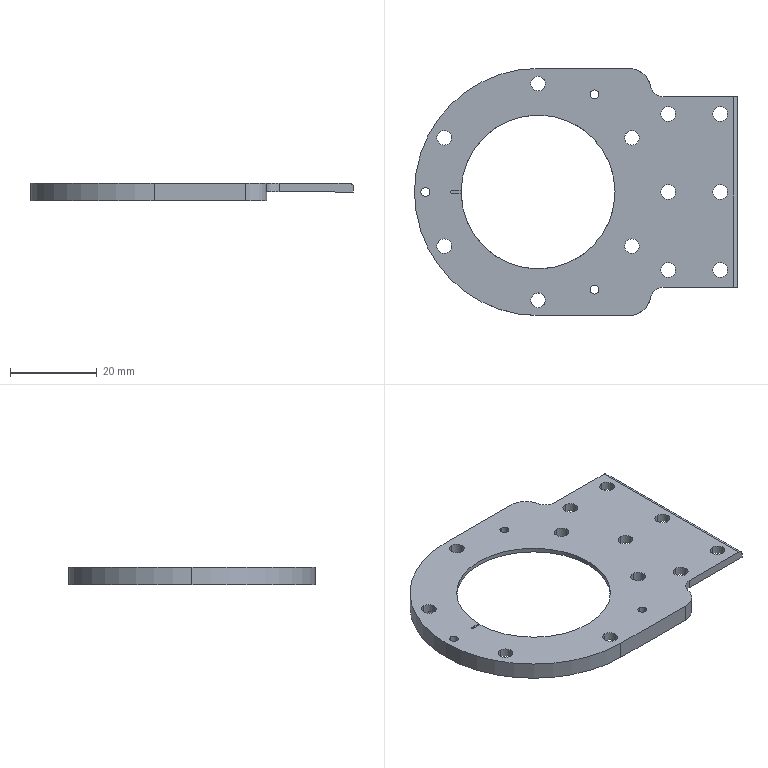NC program | NX | posted with a generic post | part box 74.5 x 57 x 4 mm
Lines 1525 to 3557 of 3557, first 1751 of 2029 lines:
(ZLEVEL_PROFILE_COPY_COPY , TOOL : D10JING)
N2994 T14 M6
N2996 G54
N2998 G17 G0 G90 X-19.345 Y1.822 S9500 M3
N3000 G43 Z30. H14
N3002 Z-3.
N3004 G94 G1 Z-4. F1000.
N3006 X-21. Y0.866
N3008 G3 X-21.5 Y0. R1.
N3010 X-8.75 Y-12.75 R12.75 F1500.
N3012 X-21.5 Y0. R-12.75
N3014 X-21. Y-0.866 R1.
N3016 G1 X-19.345 Y-1.822
N3018 Z-3.
N3020 G0 Z30.
(ZLEVEL_PROFILE_COPY , TOOL : D10JING)
N3022 X44.059 Y23.622
N3024 Z-2.525
N3026 G1 Z-3.525 F1000.
N3028 X42.75 Y22.866
N3030 G3 X42.25 Y22. R1.
N3032 G1 Y-22. F1200.
N3034 G2 X37.25 Y-27. R5.
N3036 G1 X21.617
N3038 G2 X12.25 Y-33.5 R10.
N3040 G1 X-8.75
N3042 G2 X-42.25 Y0. R33.5
N3044 X-8.75 Y33.5 R33.5
N3046 G1 X12.25
N3048 G2 X21.617 Y27. R10.
N3050 G1 X37.25
N3052 G2 X42.25 Y22. R5.
N3054 G1 Y-21.784 Z-3.546
N3056 Y-22.007
N3058 X42.245 Y-22.231
N3060 X42.229 Y-22.454
N3062 X42.204 Y-22.676
N3064 X42.169 Y-22.896
N3066 X42.124 Y-23.115
N3068 X42.069 Y-23.331 Z-3.547
N3070 X42.005 Y-23.545
N3072 X41.931 Y-23.756
N3074 X41.848 Y-23.964
N3076 X41.756 Y-24.167
N3078 X41.655 Y-24.366
N3080 X41.545 Y-24.56
N3082 X41.426 Y-24.75
N3084 X41.299 Y-24.933
N3086 X41.164 Y-25.111 Z-3.548
N3088 X41.021 Y-25.283
N3090 X40.871 Y-25.448
N3092 X40.713 Y-25.607
N3094 X40.549 Y-25.758
N3096 X40.377 Y-25.901
N3098 X40.2 Y-26.037
N3100 X40.017 Y-26.165
N3102 X39.828 Y-26.284
N3104 X39.634 Y-26.395 Z-3.549
N3106 X39.436 Y-26.497
N3108 X39.232 Y-26.59
N3110 X39.025 Y-26.674
N3112 X38.815 Y-26.749
N3114 X38.601 Y-26.814
N3116 X38.385 Y-26.869
N3118 X38.166 Y-26.915
N3120 X37.946 Y-26.951
N3122 X37.724 Y-26.977
N3124 X37.501 Y-26.994 Z-3.55
N3126 X37.278 Y-27.
N3128 X37.055
N3130 X21.641 Z-3.557
N3132 X21.546 Y-27.187
N3134 X21.461 Y-27.393
N3136 X21.372 Y-27.598
N3138 X21.278 Y-27.801 Z-3.558
N3140 X21.18 Y-28.001
N3142 X21.077 Y-28.2
N3144 X20.97 Y-28.396
N3146 X20.858 Y-28.589
N3148 X20.742 Y-28.78
N3150 X20.622 Y-28.969
N3152 X20.498 Y-29.154
N3154 X20.37 Y-29.337
N3156 X20.237 Y-29.517 Z-3.559
N3158 X20.101 Y-29.694
N3160 X19.96 Y-29.868
N3162 X19.816 Y-30.038
N3164 X19.668 Y-30.206
N3166 X19.517 Y-30.37
N3168 X19.361 Y-30.53
N3170 X19.203 Y-30.688
N3172 X19.04 Y-30.841
N3174 X18.875 Y-30.991
N3176 X18.706 Y-31.137 Z-3.56
N3178 X18.533 Y-31.279
N3180 X18.358 Y-31.418
N3182 X18.18 Y-31.552
N3184 X17.998 Y-31.683
N3186 X17.814 Y-31.809
N3188 X17.627 Y-31.931
N3190 X17.438 Y-32.049
N3192 X17.245 Y-32.163
N3194 X17.051 Y-32.272 Z-3.561
N3196 X16.853 Y-32.377
N3198 X16.654 Y-32.478
N3200 X16.452 Y-32.574
N3202 X16.249 Y-32.666
N3204 X16.043 Y-32.753
N3206 X15.835 Y-32.835
N3208 X15.626 Y-32.913
N3210 X15.415 Y-32.986
N3212 X15.202 Y-33.054
N3214 X14.988 Y-33.118 Z-3.562
N3216 X14.772 Y-33.177
N3218 X14.556 Y-33.231
N3220 X14.338 Y-33.28
N3222 X14.119 Y-33.324
N3224 X13.899 Y-33.363
N3226 X13.678 Y-33.398
N3228 X13.457 Y-33.427
N3230 X13.235 Y-33.451
N3232 X13.012 Y-33.471 Z-3.563
N3234 X12.789 Y-33.485
N3236 X12.566 Y-33.495
N3238 X12.343 Y-33.5
N3240 X12.119
N3242 X-8.656 Z-3.573
N3244 X-8.879
N3246 X-9.103 Y-33.498
N3248 X-9.326 Y-33.495
N3250 X-9.549 Y-33.49
N3252 X-9.773 Y-33.484
N3254 X-9.996 Y-33.477 Z-3.574
N3256 X-10.219 Y-33.468
N3258 X-10.442 Y-33.457
N3260 X-10.665 Y-33.445
N3262 X-10.888 Y-33.432
N3264 X-11.111 Y-33.417
N3266 X-11.334 Y-33.4
N3268 X-11.557 Y-33.382
N3270 X-11.779 Y-33.363
N3272 X-12.002 Y-33.342
N3274 X-12.224 Y-33.319 Z-3.575
N3276 X-12.446 Y-33.296
N3278 X-12.668 Y-33.27
N3280 X-12.89 Y-33.243
N3282 X-13.111 Y-33.215
N3284 X-13.333 Y-33.185
N3286 X-13.554 Y-33.154
N3288 X-13.775 Y-33.121
N3290 X-13.995 Y-33.087
N3292 X-14.216 Y-33.051 Z-3.576
N3294 X-14.436 Y-33.014
N3296 X-14.656 Y-32.975
N3298 X-14.876 Y-32.935
N3300 X-15.096 Y-32.894
N3302 X-15.315 Y-32.85
N3304 X-15.534 Y-32.806
N3306 X-15.752 Y-32.76
N3308 X-15.971 Y-32.713
N3310 X-16.189 Y-32.664
N3312 X-16.406 Y-32.613 Z-3.577
N3314 X-16.623 Y-32.562
N3316 X-16.84 Y-32.508
N3318 X-17.057 Y-32.454
N3320 X-17.273 Y-32.398
N3322 X-17.489 Y-32.34
N3324 X-17.705 Y-32.281
N3326 X-17.92 Y-32.221
N3328 X-18.134 Y-32.159
N3330 X-18.348 Y-32.095 Z-3.578
N3332 X-18.562 Y-32.031
N3334 X-18.776 Y-31.965
N3336 X-18.989 Y-31.897
N3338 X-19.201 Y-31.828
N3340 X-19.413 Y-31.758
N3342 X-19.625 Y-31.686
N3344 X-19.836 Y-31.613
N3346 X-20.046 Y-31.538
N3348 X-20.256 Y-31.462 Z-3.579
N3350 X-20.466 Y-31.385
N3352 X-20.675 Y-31.306
N3354 X-20.883 Y-31.226
N3356 X-21.091 Y-31.144
N3358 X-21.299 Y-31.061
N3360 X-21.505 Y-30.977
N3362 X-21.712 Y-30.891
N3364 X-21.917 Y-30.804
N3366 X-22.123 Y-30.715
N3368 X-22.327 Y-30.625 Z-3.58
N3370 X-22.531 Y-30.534
N3372 X-22.734 Y-30.442
N3374 X-22.937 Y-30.348
N3376 X-23.139 Y-30.252
N3378 X-23.34 Y-30.156
N3380 X-23.541 Y-30.058
N3382 X-23.741 Y-29.958
N3384 X-23.941 Y-29.858
N3386 X-24.14 Y-29.756 Z-3.581
N3388 X-24.338 Y-29.653
N3390 X-24.535 Y-29.548
N3392 X-24.732 Y-29.442
N3394 X-24.928 Y-29.335
N3396 X-25.123 Y-29.226
N3398 X-25.317 Y-29.117
N3400 X-25.511 Y-29.005
N3402 X-25.704 Y-28.893
N3404 X-25.897 Y-28.779
N3406 X-26.088 Y-28.664 Z-3.582
N3408 X-26.279 Y-28.548
N3410 X-26.469 Y-28.431
N3412 X-26.658 Y-28.312
N3414 X-26.846 Y-28.192
N3416 X-27.034 Y-28.07
N3418 X-27.221 Y-27.948
N3420 X-27.407 Y-27.824
N3422 X-27.592 Y-27.699
N3424 X-27.776 Y-27.573 Z-3.583
N3426 X-27.96 Y-27.445
N3428 X-28.142 Y-27.317
N3430 X-28.324 Y-27.187
N3432 X-28.505 Y-27.056
N3434 X-28.685 Y-26.923
N3436 X-28.864 Y-26.79
N3438 X-29.042 Y-26.655
N3440 X-29.219 Y-26.519
N3442 X-29.396 Y-26.382 Z-3.584
N3444 X-29.571 Y-26.244
N3446 X-29.746 Y-26.104
N3448 X-29.919 Y-25.964
N3450 X-30.092 Y-25.822
N3452 X-30.264 Y-25.679
N3454 X-30.434 Y-25.535
N3456 X-30.604 Y-25.39
N3458 X-30.773 Y-25.244
N3460 X-30.941 Y-25.096
N3462 X-31.108 Y-24.948 Z-3.585
N3464 X-31.274 Y-24.798
N3466 X-31.438 Y-24.647
N3468 X-31.602 Y-24.495
N3470 X-31.765 Y-24.343
N3472 X-31.927 Y-24.188
N3474 X-32.088 Y-24.033
N3476 X-32.247 Y-23.877
N3478 X-32.406 Y-23.72
N3480 X-32.564 Y-23.562 Z-3.586
N3482 X-32.72 Y-23.402
N3484 X-32.876 Y-23.242
N3486 X-33.03 Y-23.081
N3488 X-33.184 Y-22.918
N3490 X-33.336 Y-22.755
N3492 X-33.487 Y-22.59
N3494 X-33.637 Y-22.425
N3496 X-33.786 Y-22.258
N3498 X-33.934 Y-22.091
N3500 X-34.081 Y-21.923 Z-3.587
N3502 X-34.226 Y-21.753
N3504 X-34.371 Y-21.583
N3506 X-34.514 Y-21.412
N3508 X-34.656 Y-21.239
N3510 X-34.798 Y-21.066
N3512 X-34.937 Y-20.892
N3514 X-35.076 Y-20.717
N3516 X-35.214 Y-20.541
N3518 X-35.35 Y-20.364 Z-3.588
N3520 X-35.485 Y-20.186
N3522 X-35.619 Y-20.007
N3524 X-35.752 Y-19.828
N3526 X-35.884 Y-19.647
N3528 X-36.014 Y-19.466
N3530 X-36.143 Y-19.284
N3532 X-36.271 Y-19.1
N3534 X-36.398 Y-18.917
N3536 X-36.524 Y-18.732 Z-3.589
N3538 X-36.648 Y-18.546
N3540 X-36.771 Y-18.36
N3542 X-36.893 Y-18.172
N3544 X-37.013 Y-17.984
N3546 X-37.133 Y-17.795
N3548 X-37.251 Y-17.606
N3550 X-37.367 Y-17.415
N3552 X-37.483 Y-17.224
N3554 X-37.597 Y-17.032
N3556 X-37.71 Y-16.839 Z-3.59
N3558 X-37.822 Y-16.646
N3560 X-37.932 Y-16.452
N3562 X-38.041 Y-16.257
N3564 X-38.149 Y-16.061
N3566 X-38.255 Y-15.865
N3568 X-38.36 Y-15.668
N3570 X-38.464 Y-15.47
N3572 X-38.567 Y-15.271
N3574 X-38.668 Y-15.072 Z-3.591
N3576 X-38.768 Y-14.872
N3578 X-38.866 Y-14.672
N3580 X-38.963 Y-14.471
N3582 X-39.059 Y-14.269
N3584 X-39.154 Y-14.066
N3586 X-39.247 Y-13.863
N3588 X-39.339 Y-13.66
N3590 X-39.429 Y-13.455
N3592 X-39.518 Y-13.251
N3594 X-39.606 Y-13.045 Z-3.592
N3596 X-39.692 Y-12.839
N3598 X-39.777 Y-12.632
N3600 X-39.86 Y-12.425
N3602 X-39.943 Y-12.218
N3604 X-40.023 Y-12.009
N3606 X-40.103 Y-11.8
N3608 X-40.181 Y-11.591
N3610 X-40.257 Y-11.381
N3612 X-40.333 Y-11.171 Z-3.593
N3614 X-40.406 Y-10.96
N3616 X-40.479 Y-10.749
N3618 X-40.55 Y-10.537
N3620 X-40.619 Y-10.325
N3622 X-40.687 Y-10.112
N3624 X-40.754 Y-9.899
N3626 X-40.819 Y-9.685
N3628 X-40.883 Y-9.471
N3630 X-40.946 Y-9.257 Z-3.594
N3632 X-41.007 Y-9.042
N3634 X-41.066 Y-8.826
N3636 X-41.124 Y-8.611
N3638 X-41.181 Y-8.395
N3640 X-41.236 Y-8.178
N3642 X-41.29 Y-7.961
N3644 X-41.343 Y-7.744
N3646 X-41.394 Y-7.527
N3648 X-41.443 Y-7.309
N3650 X-41.491 Y-7.091 Z-3.595
N3652 X-41.538 Y-6.872
N3654 X-41.583 Y-6.653
N3656 X-41.626 Y-6.434
N3658 X-41.668 Y-6.215
N3660 X-41.709 Y-5.995
N3662 X-41.748 Y-5.775
N3664 X-41.786 Y-5.555
N3666 X-41.822 Y-5.335
N3668 X-41.857 Y-5.114 Z-3.596
N3670 X-41.891 Y-4.893
N3672 X-41.923 Y-4.672
N3674 X-41.953 Y-4.451
N3676 X-41.982 Y-4.229
N3678 X-42.009 Y-4.008
N3680 X-42.035 Y-3.786
N3682 X-42.06 Y-3.564
N3684 X-42.083 Y-3.342
N3686 X-42.104 Y-3.119
N3688 X-42.125 Y-2.897 Z-3.597
N3690 X-42.143 Y-2.674
N3692 X-42.16 Y-2.451
N3694 X-42.176 Y-2.229
N3696 X-42.19 Y-2.006
N3698 X-42.203 Y-1.783
N3700 X-42.214 Y-1.559
N3702 X-42.223 Y-1.336
N3704 X-42.232 Y-1.113
N3706 X-42.238 Y-0.89 Z-3.598
N3708 X-42.243 Y-0.666
N3710 X-42.247 Y-0.443
N3712 X-42.249 Y-0.22
N3714 X-42.25 Y0.004
N3716 X-42.249 Y0.227
N3718 X-42.247 Y0.45
N3720 X-42.243 Y0.674
N3722 X-42.238 Y0.897
N3724 X-42.231 Y1.12 Z-3.599
N3726 X-42.223 Y1.344
N3728 X-42.213 Y1.567
N3730 X-42.202 Y1.79
N3732 X-42.189 Y2.013
N3734 X-42.175 Y2.236
N3736 X-42.16 Y2.459
N3738 X-42.143 Y2.681
N3740 X-42.124 Y2.904
N3742 X-42.104 Y3.127
N3744 X-42.082 Y3.349 Z-3.6
N3746 X-42.059 Y3.571
N3748 X-42.035 Y3.793
N3750 X-42.009 Y4.015
N3752 X-41.981 Y4.237
N3754 X-41.952 Y4.458
N3756 X-41.922 Y4.68
N3758 X-41.89 Y4.901
N3760 X-41.856 Y5.121
N3762 X-41.821 Y5.342 Z-3.601
N3764 X-41.785 Y5.563
N3766 X-41.747 Y5.783
N3768 X-41.708 Y6.003
N3770 X-41.667 Y6.222
N3772 X-41.625 Y6.442
N3774 X-41.581 Y6.661
N3776 X-41.536 Y6.879
N3778 X-41.489 Y7.098
N3780 X-41.441 Y7.316
N3782 X-41.392 Y7.534 Z-3.602
N3784 X-41.341 Y7.751
N3786 X-41.288 Y7.969
N3788 X-41.235 Y8.185
N3790 X-41.179 Y8.402
N3792 X-41.123 Y8.618
N3794 X-41.064 Y8.834
N3796 X-41.005 Y9.049
N3798 X-40.944 Y9.264
N3800 X-40.881 Y9.478 Z-3.603
N3802 X-40.817 Y9.692
N3804 X-40.752 Y9.906
N3806 X-40.685 Y10.119
N3808 X-40.617 Y10.332
N3810 X-40.547 Y10.544
N3812 X-40.476 Y10.756
N3814 X-40.404 Y10.967
N3816 X-40.33 Y11.178
N3818 X-40.255 Y11.388 Z-3.604
N3820 X-40.178 Y11.598
N3822 X-40.1 Y11.807
N3824 X-40.021 Y12.016
N3826 X-39.94 Y12.224
N3828 X-39.858 Y12.432
N3830 X-39.774 Y12.639
N3832 X-39.689 Y12.846
N3834 X-39.603 Y13.052
N3836 X-39.515 Y13.257
N3838 X-39.426 Y13.462 Z-3.605
N3840 X-39.336 Y13.667
N3842 X-39.244 Y13.87
N3844 X-39.151 Y14.073
N3846 X-39.056 Y14.276
N3848 X-38.96 Y14.477
N3850 X-38.863 Y14.678
N3852 X-38.764 Y14.879
N3854 X-38.665 Y15.079
N3856 X-38.563 Y15.278 Z-3.606
N3858 X-38.461 Y15.476
N3860 X-38.357 Y15.674
N3862 X-38.252 Y15.871
N3864 X-38.145 Y16.068
N3866 X-38.037 Y16.263
N3868 X-37.928 Y16.458
N3870 X-37.818 Y16.652
N3872 X-37.706 Y16.846
N3874 X-37.593 Y17.039
N3876 X-37.479 Y17.231 Z-3.607
N3878 X-37.364 Y17.422
N3880 X-37.247 Y17.612
N3882 X-37.129 Y17.802
N3884 X-37.009 Y17.991
N3886 X-36.889 Y18.179
N3888 X-36.767 Y18.366
N3890 X-36.644 Y18.552
N3892 X-36.519 Y18.738
N3894 X-36.394 Y18.923 Z-3.608
N3896 X-36.267 Y19.107
N3898 X-36.139 Y19.29
N3900 X-36.01 Y19.472
N3902 X-35.879 Y19.653
N3904 X-35.748 Y19.834
N3906 X-35.615 Y20.013
N3908 X-35.481 Y20.192
N3910 X-35.346 Y20.37
N3912 X-35.209 Y20.547 Z-3.609
N3914 X-35.072 Y20.723
N3916 X-34.933 Y20.898
N3918 X-34.793 Y21.072
N3920 X-34.652 Y21.245
N3922 X-34.51 Y21.417
N3924 X-34.366 Y21.589
N3926 X-34.222 Y21.759
N3928 X-34.076 Y21.928
N3930 X-33.929 Y22.097
N3932 X-33.781 Y22.264 Z-3.61
N3934 X-33.632 Y22.43
N3936 X-33.482 Y22.596
N3938 X-33.331 Y22.76
N3940 X-33.179 Y22.924
N3942 X-33.025 Y23.086
N3944 X-32.871 Y23.247
N3946 X-32.715 Y23.408
N3948 X-32.558 Y23.567
N3950 X-32.401 Y23.725 Z-3.611
N3952 X-32.242 Y23.882
N3954 X-32.082 Y24.039
N3956 X-31.921 Y24.194
N3958 X-31.76 Y24.348
N3960 X-31.597 Y24.5
N3962 X-31.433 Y24.652
N3964 X-31.268 Y24.803
N3966 X-31.102 Y24.953
N3968 X-30.935 Y25.101
N3970 X-30.767 Y25.248 Z-3.612
N3972 X-30.599 Y25.395
N3974 X-30.429 Y25.54
N3976 X-30.258 Y25.684
N3978 X-30.086 Y25.827
N3980 X-29.913 Y25.968
N3982 X-29.74 Y26.109
N3984 X-29.565 Y26.248
N3986 X-29.39 Y26.387
N3988 X-29.213 Y26.524 Z-3.613
N3990 X-29.036 Y26.659
N3992 X-28.858 Y26.794
N3994 X-28.679 Y26.928
N3996 X-28.499 Y27.06
N3998 X-28.318 Y27.191
N4000 X-28.136 Y27.321
N4002 X-27.953 Y27.45
N4004 X-27.77 Y27.577
N4006 X-27.586 Y27.703 Z-3.614
N4008 X-27.401 Y27.828
N4010 X-27.215 Y27.952
N4012 X-27.028 Y28.074
N4014 X-26.84 Y28.196
N4016 X-26.652 Y28.316
N4018 X-26.462 Y28.434
N4020 X-26.272 Y28.552
N4022 X-26.082 Y28.668
N4024 X-25.89 Y28.783
N4026 X-25.698 Y28.897 Z-3.615
N4028 X-25.505 Y29.009
N4030 X-25.311 Y29.12
N4032 X-25.116 Y29.23
N4034 X-24.921 Y29.338
N4036 X-24.725 Y29.446
N4038 X-24.528 Y29.552
N4040 X-24.331 Y29.656
N4042 X-24.133 Y29.759
N4044 X-23.934 Y29.861 Z-3.616
N4046 X-23.735 Y29.962
N4048 X-23.535 Y30.061
N4050 X-23.334 Y30.159
N4052 X-23.132 Y30.256
N4054 X-22.93 Y30.351
N4056 X-22.728 Y30.445
N4058 X-22.524 Y30.537
N4060 X-22.32 Y30.628
N4062 X-22.116 Y30.718
N4064 X-21.911 Y30.807 Z-3.617
N4066 X-21.705 Y30.894
N4068 X-21.499 Y30.979
N4070 X-21.292 Y31.064
N4072 X-21.084 Y31.147
N4074 X-20.876 Y31.228
N4076 X-20.668 Y31.308
N4078 X-20.459 Y31.387
N4080 X-20.249 Y31.465
N4082 X-20.039 Y31.541 Z-3.618
N4084 X-19.829 Y31.615
N4086 X-19.618 Y31.688
N4088 X-19.406 Y31.76
N4090 X-19.194 Y31.83
N4092 X-18.982 Y31.899
N4094 X-18.769 Y31.967
N4096 X-18.555 Y32.033
N4098 X-18.341 Y32.098
N4100 X-18.127 Y32.161 Z-3.619
N4102 X-17.912 Y32.223
N4104 X-17.697 Y32.283
N4106 X-17.482 Y32.342
N4108 X-17.266 Y32.399
N4110 X-17.05 Y32.456
N4112 X-16.833 Y32.51
N4114 X-16.616 Y32.563
N4116 X-16.399 Y32.615
N4118 X-16.181 Y32.665
N4120 X-15.963 Y32.714 Z-3.62
N4122 X-15.745 Y32.762
N4124 X-15.526 Y32.807
N4126 X-15.307 Y32.852
N4128 X-15.088 Y32.895
N4130 X-14.869 Y32.936
N4132 X-14.649 Y32.977
N4134 X-14.429 Y33.015
N4136 X-14.209 Y33.052
N4138 X-13.988 Y33.088 Z-3.621
N4140 X-13.767 Y33.122
N4142 X-13.546 Y33.155
N4144 X-13.325 Y33.186
N4146 X-13.104 Y33.216
N4148 X-12.882 Y33.244
N4150 X-12.66 Y33.271
N4152 X-12.439 Y33.296
N4154 X-12.216 Y33.32
N4156 X-11.994 Y33.343
N4158 X-11.772 Y33.363 Z-3.622
N4160 X-11.549 Y33.383
N4162 X-11.327 Y33.401
N4164 X-11.104 Y33.417
N4166 X-10.881 Y33.432
N4168 X-10.658 Y33.446
N4170 X-10.435 Y33.458
N4172 X-10.212 Y33.468
N4174 X-9.988 Y33.477
N4176 X-9.765 Y33.485 Z-3.623
N4178 X-9.542 Y33.491
N4180 X-9.319 Y33.495
N4182 X-9.095 Y33.498
N4184 X-8.872 Y33.5
N4186 X-8.648
N4188 X12.127 Z-3.633
N4190 X12.35
N4192 X12.573 Y33.495
N4194 X12.797 Y33.485
N4196 X13.019 Y33.47
N4198 X13.242 Y33.451 Z-3.634
N4200 X13.464 Y33.426
N4202 X13.685 Y33.396
N4204 X13.906 Y33.362
N4206 X14.126 Y33.322
N4208 X14.345 Y33.278
N4210 X14.563 Y33.229
N4212 X14.78 Y33.175
N4214 X14.995 Y33.116
N4216 X15.209 Y33.052
N4218 X15.422 Y32.984 Z-3.635
N4220 X15.633 Y32.91
N4222 X15.842 Y32.833
N4224 X16.05 Y32.75
N4226 X16.255 Y32.663
N4228 X16.459 Y32.571
N4230 X16.661 Y32.475
N4232 X16.86 Y32.374
N4234 X17.057 Y32.269
N4236 X17.252 Y32.159 Z-3.636
N4238 X17.444 Y32.045
N4240 X17.633 Y31.927
N4242 X17.82 Y31.805
N4244 X18.004 Y31.678
N4246 X18.186 Y31.548
N4248 X18.364 Y31.413
N4250 X18.539 Y31.275
N4252 X18.711 Y31.132
N4254 X18.88 Y30.986
N4256 X19.046 Y30.836 Z-3.637
N4258 X19.208 Y30.682
N4260 X19.367 Y30.525
N4262 X19.522 Y30.364
N4264 X19.673 Y30.2
N4266 X19.821 Y30.033
N4268 X19.965 Y29.862
N4270 X20.105 Y29.688
N4272 X20.242 Y29.511
N4274 X20.374 Y29.331 Z-3.638
N4276 X20.502 Y29.148
N4278 X20.626 Y28.963
N4280 X20.746 Y28.774
N4282 X20.862 Y28.583
N4284 X20.973 Y28.389
N4286 X21.08 Y28.193
N4288 X21.183 Y27.995
N4290 X21.281 Y27.794
N4292 X21.375 Y27.591 Z-3.639
N4294 X21.464 Y27.387
N4296 X21.548 Y27.18
N4298 X21.648 Y27.
N4300 X37.062 Z-3.646
N4302 X37.285
N4304 X37.509 Y26.993
N4306 X37.731 Y26.977
N4308 X37.953 Y26.95 Z-3.647
N4310 X38.174 Y26.914
N4312 X38.392 Y26.868
N4314 X38.608 Y26.812
N4316 X38.822 Y26.746
N4318 X39.032 Y26.672
N4320 X39.239 Y26.587
N4322 X39.442 Y26.494
N4324 X39.641 Y26.391
N4326 X39.834 Y26.28 Z-3.648
N4328 X40.023 Y26.161
N4330 X40.206 Y26.033
N4332 X40.383 Y25.897
N4334 X40.554 Y25.753
N4336 X40.718 Y25.601
N4338 X40.876 Y25.443
N4340 X41.026 Y25.277
N4342 X41.169 Y25.106
N4344 X41.303 Y24.927 Z-3.649
N4346 X41.43 Y24.744
N4348 X41.548 Y24.554
N4350 X41.658 Y24.36
N4352 X41.759 Y24.16
N4354 X41.851 Y23.957
N4356 X41.934 Y23.749
N4358 X42.007 Y23.538
N4360 X42.071 Y23.324
N4362 X42.126 Y23.108
N4364 X42.17 Y22.889 Z-3.65
N4366 X42.205 Y22.668
N4368 X42.23 Y22.446
N4370 X42.245 Y22.223
N4372 X42.25 Y22.
N4374 Y-21.784 Z-3.671
N4376 Y-22.007
N4378 X42.245 Y-22.231
N4380 X42.229 Y-22.454
N4382 X42.204 Y-22.676
N4384 X42.169 Y-22.896
N4386 X42.124 Y-23.115
N4388 X42.069 Y-23.331 Z-3.672
N4390 X42.005 Y-23.545
N4392 X41.931 Y-23.756
N4394 X41.848 Y-23.964
N4396 X41.756 Y-24.167
N4398 X41.655 Y-24.366
N4400 X41.545 Y-24.56
N4402 X41.426 Y-24.75
N4404 X41.299 Y-24.933
N4406 X41.164 Y-25.111 Z-3.673
N4408 X41.021 Y-25.283
N4410 X40.871 Y-25.448
N4412 X40.713 Y-25.607
N4414 X40.549 Y-25.758
N4416 X40.377 Y-25.901
N4418 X40.2 Y-26.037
N4420 X40.017 Y-26.165
N4422 X39.828 Y-26.284
N4424 X39.634 Y-26.395 Z-3.674
N4426 X39.436 Y-26.497
N4428 X39.232 Y-26.59
N4430 X39.025 Y-26.674
N4432 X38.815 Y-26.749
N4434 X38.601 Y-26.814
N4436 X38.385 Y-26.869
N4438 X38.166 Y-26.915
N4440 X37.946 Y-26.951
N4442 X37.724 Y-26.977
N4444 X37.501 Y-26.994 Z-3.675
N4446 X37.278 Y-27.
N4448 X37.055
N4450 X21.641 Z-3.682
N4452 X21.546 Y-27.187
N4454 X21.461 Y-27.393
N4456 X21.372 Y-27.598
N4458 X21.278 Y-27.801 Z-3.683
N4460 X21.18 Y-28.001
N4462 X21.077 Y-28.2
N4464 X20.97 Y-28.396
N4466 X20.858 Y-28.589
N4468 X20.742 Y-28.78
N4470 X20.622 Y-28.969
N4472 X20.498 Y-29.154
N4474 X20.37 Y-29.337
N4476 X20.237 Y-29.517 Z-3.684
N4478 X20.101 Y-29.694
N4480 X19.96 Y-29.868
N4482 X19.816 Y-30.038
N4484 X19.668 Y-30.206
N4486 X19.517 Y-30.37
N4488 X19.361 Y-30.53
N4490 X19.203 Y-30.688
N4492 X19.04 Y-30.841
N4494 X18.875 Y-30.991
N4496 X18.706 Y-31.137 Z-3.685
N4498 X18.533 Y-31.279
N4500 X18.358 Y-31.418
N4502 X18.18 Y-31.552
N4504 X17.998 Y-31.683
N4506 X17.814 Y-31.809
N4508 X17.627 Y-31.931
N4510 X17.438 Y-32.049
N4512 X17.245 Y-32.163
N4514 X17.051 Y-32.272 Z-3.686
N4516 X16.853 Y-32.377
N4518 X16.654 Y-32.478
N4520 X16.452 Y-32.574
N4522 X16.249 Y-32.666
N4524 X16.043 Y-32.753
N4526 X15.835 Y-32.835
N4528 X15.626 Y-32.913
N4530 X15.415 Y-32.986
N4532 X15.202 Y-33.054
N4534 X14.988 Y-33.118 Z-3.687
N4536 X14.772 Y-33.177
N4538 X14.556 Y-33.231
N4540 X14.338 Y-33.28
N4542 X14.119 Y-33.324
N4544 X13.899 Y-33.363
N4546 X13.678 Y-33.398
N4548 X13.457 Y-33.427
N4550 X13.235 Y-33.451
N4552 X13.012 Y-33.471 Z-3.688
N4554 X12.789 Y-33.485
N4556 X12.566 Y-33.495
N4558 X12.343 Y-33.5
N4560 X12.119
N4562 X-8.656 Z-3.698
N4564 X-8.879
N4566 X-9.103 Y-33.498
N4568 X-9.326 Y-33.495
N4570 X-9.549 Y-33.49
N4572 X-9.773 Y-33.484
N4574 X-9.996 Y-33.477 Z-3.699
N4576 X-10.219 Y-33.468
N4578 X-10.442 Y-33.457
N4580 X-10.665 Y-33.445
N4582 X-10.888 Y-33.432
N4584 X-11.111 Y-33.417
N4586 X-11.334 Y-33.4
N4588 X-11.557 Y-33.382
N4590 X-11.779 Y-33.363
N4592 X-12.002 Y-33.342
N4594 X-12.224 Y-33.319 Z-3.7
N4596 X-12.446 Y-33.296
N4598 X-12.668 Y-33.27
N4600 X-12.89 Y-33.243
N4602 X-13.111 Y-33.215
N4604 X-13.333 Y-33.185
N4606 X-13.554 Y-33.154
N4608 X-13.775 Y-33.121
N4610 X-13.995 Y-33.087
N4612 X-14.216 Y-33.051 Z-3.701
N4614 X-14.436 Y-33.014
N4616 X-14.656 Y-32.975
N4618 X-14.876 Y-32.935
N4620 X-15.096 Y-32.894
N4622 X-15.315 Y-32.85
N4624 X-15.534 Y-32.806
N4626 X-15.752 Y-32.76
N4628 X-15.971 Y-32.713
N4630 X-16.189 Y-32.664
N4632 X-16.406 Y-32.613 Z-3.702
N4634 X-16.623 Y-32.562
N4636 X-16.84 Y-32.508
N4638 X-17.057 Y-32.454
N4640 X-17.273 Y-32.398
N4642 X-17.489 Y-32.34
N4644 X-17.705 Y-32.281
N4646 X-17.92 Y-32.221
N4648 X-18.134 Y-32.159
N4650 X-18.348 Y-32.095 Z-3.703
N4652 X-18.562 Y-32.031
N4654 X-18.776 Y-31.965
N4656 X-18.989 Y-31.897
N4658 X-19.201 Y-31.828
N4660 X-19.413 Y-31.758
N4662 X-19.625 Y-31.686
N4664 X-19.836 Y-31.613
N4666 X-20.046 Y-31.538
N4668 X-20.256 Y-31.462 Z-3.704
N4670 X-20.466 Y-31.385
N4672 X-20.675 Y-31.306
N4674 X-20.883 Y-31.226
N4676 X-21.091 Y-31.144
N4678 X-21.299 Y-31.061
N4680 X-21.505 Y-30.977
N4682 X-21.712 Y-30.891
N4684 X-21.917 Y-30.804
N4686 X-22.123 Y-30.715
N4688 X-22.327 Y-30.625 Z-3.705
N4690 X-22.531 Y-30.534
N4692 X-22.734 Y-30.442
N4694 X-22.937 Y-30.348
N4696 X-23.139 Y-30.252
N4698 X-23.34 Y-30.156
N4700 X-23.541 Y-30.058
N4702 X-23.741 Y-29.958
N4704 X-23.941 Y-29.858
N4706 X-24.14 Y-29.756 Z-3.706
N4708 X-24.338 Y-29.653
N4710 X-24.535 Y-29.548
N4712 X-24.732 Y-29.442
N4714 X-24.928 Y-29.335
N4716 X-25.123 Y-29.226
N4718 X-25.317 Y-29.117
N4720 X-25.511 Y-29.005
N4722 X-25.704 Y-28.893
N4724 X-25.897 Y-28.779
N4726 X-26.088 Y-28.664 Z-3.707
N4728 X-26.279 Y-28.548
N4730 X-26.469 Y-28.431
N4732 X-26.658 Y-28.312
N4734 X-26.846 Y-28.192
N4736 X-27.034 Y-28.07
N4738 X-27.221 Y-27.948
N4740 X-27.407 Y-27.824
N4742 X-27.592 Y-27.699
N4744 X-27.776 Y-27.573 Z-3.708
N4746 X-27.96 Y-27.445
N4748 X-28.142 Y-27.317
N4750 X-28.324 Y-27.187
N4752 X-28.505 Y-27.056
N4754 X-28.685 Y-26.923
N4756 X-28.864 Y-26.79
N4758 X-29.042 Y-26.655
N4760 X-29.219 Y-26.519
N4762 X-29.396 Y-26.382 Z-3.709
N4764 X-29.571 Y-26.244
N4766 X-29.746 Y-26.104
N4768 X-29.919 Y-25.964
N4770 X-30.092 Y-25.822
N4772 X-30.264 Y-25.679
N4774 X-30.434 Y-25.535
N4776 X-30.604 Y-25.39
N4778 X-30.773 Y-25.244
N4780 X-30.941 Y-25.096
N4782 X-31.108 Y-24.948 Z-3.71
N4784 X-31.274 Y-24.798
N4786 X-31.438 Y-24.647
N4788 X-31.602 Y-24.495
N4790 X-31.765 Y-24.343
N4792 X-31.927 Y-24.188
N4794 X-32.088 Y-24.033
N4796 X-32.247 Y-23.877
N4798 X-32.406 Y-23.72
N4800 X-32.564 Y-23.562 Z-3.711
N4802 X-32.72 Y-23.402
N4804 X-32.876 Y-23.242
N4806 X-33.03 Y-23.081
N4808 X-33.184 Y-22.918
N4810 X-33.336 Y-22.755
N4812 X-33.487 Y-22.59
N4814 X-33.637 Y-22.425
N4816 X-33.786 Y-22.258
N4818 X-33.934 Y-22.091
N4820 X-34.081 Y-21.923 Z-3.712
N4822 X-34.226 Y-21.753
N4824 X-34.371 Y-21.583
N4826 X-34.514 Y-21.412
N4828 X-34.656 Y-21.239
N4830 X-34.798 Y-21.066
N4832 X-34.937 Y-20.892
N4834 X-35.076 Y-20.717
N4836 X-35.214 Y-20.541
N4838 X-35.35 Y-20.364 Z-3.713
N4840 X-35.485 Y-20.186
N4842 X-35.619 Y-20.007
N4844 X-35.752 Y-19.828
N4846 X-35.884 Y-19.647
N4848 X-36.014 Y-19.466
N4850 X-36.143 Y-19.284
N4852 X-36.271 Y-19.1
N4854 X-36.398 Y-18.917
N4856 X-36.524 Y-18.732 Z-3.714
N4858 X-36.648 Y-18.546
N4860 X-36.771 Y-18.36
N4862 X-36.893 Y-18.172
N4864 X-37.013 Y-17.984
N4866 X-37.133 Y-17.795
N4868 X-37.251 Y-17.606
N4870 X-37.367 Y-17.415
N4872 X-37.483 Y-17.224
N4874 X-37.597 Y-17.032
N4876 X-37.71 Y-16.839 Z-3.715
N4878 X-37.822 Y-16.646
N4880 X-37.932 Y-16.452
N4882 X-38.041 Y-16.257
N4884 X-38.149 Y-16.061
N4886 X-38.255 Y-15.865
N4888 X-38.36 Y-15.668
N4890 X-38.464 Y-15.47
N4892 X-38.567 Y-15.271
N4894 X-38.668 Y-15.072 Z-3.716
N4896 X-38.768 Y-14.872
N4898 X-38.866 Y-14.672
N4900 X-38.963 Y-14.471
N4902 X-39.059 Y-14.269
N4904 X-39.154 Y-14.066
N4906 X-39.247 Y-13.863
N4908 X-39.339 Y-13.66
N4910 X-39.429 Y-13.455
N4912 X-39.518 Y-13.251
N4914 X-39.606 Y-13.045 Z-3.717
N4916 X-39.692 Y-12.839
N4918 X-39.777 Y-12.632
N4920 X-39.86 Y-12.425
N4922 X-39.943 Y-12.218
N4924 X-40.023 Y-12.009
N4926 X-40.103 Y-11.8
N4928 X-40.181 Y-11.591
N4930 X-40.257 Y-11.381
N4932 X-40.333 Y-11.171 Z-3.718
N4934 X-40.406 Y-10.96
N4936 X-40.479 Y-10.749
N4938 X-40.55 Y-10.537
N4940 X-40.619 Y-10.325
N4942 X-40.687 Y-10.112
N4944 X-40.754 Y-9.899
N4946 X-40.819 Y-9.685
N4948 X-40.883 Y-9.471
N4950 X-40.946 Y-9.257 Z-3.719
N4952 X-41.007 Y-9.042
N4954 X-41.066 Y-8.826
N4956 X-41.124 Y-8.611
N4958 X-41.181 Y-8.395
N4960 X-41.236 Y-8.178
N4962 X-41.29 Y-7.961
N4964 X-41.343 Y-7.744
N4966 X-41.394 Y-7.527
N4968 X-41.443 Y-7.309
N4970 X-41.491 Y-7.091 Z-3.72
N4972 X-41.538 Y-6.872
N4974 X-41.583 Y-6.653
N4976 X-41.626 Y-6.434
N4978 X-41.668 Y-6.215
N4980 X-41.709 Y-5.995
N4982 X-41.748 Y-5.775
N4984 X-41.786 Y-5.555
N4986 X-41.822 Y-5.335
N4988 X-41.857 Y-5.114 Z-3.721
N4990 X-41.891 Y-4.893
N4992 X-41.923 Y-4.672
N4994 X-41.953 Y-4.451
N4996 X-41.982 Y-4.229
N4998 X-42.009 Y-4.008
N5000 X-42.035 Y-3.786
N5002 X-42.06 Y-3.564
N5004 X-42.083 Y-3.342
N5006 X-42.104 Y-3.119
N5008 X-42.125 Y-2.897 Z-3.722
N5010 X-42.143 Y-2.674
N5012 X-42.16 Y-2.451
N5014 X-42.176 Y-2.229
N5016 X-42.19 Y-2.006
N5018 X-42.203 Y-1.783
N5020 X-42.214 Y-1.559
N5022 X-42.223 Y-1.336
N5024 X-42.232 Y-1.113
N5026 X-42.238 Y-0.89 Z-3.723
N5028 X-42.243 Y-0.666
N5030 X-42.247 Y-0.443
N5032 X-42.249 Y-0.22
N5034 X-42.25 Y0.004
N5036 X-42.249 Y0.227
N5038 X-42.247 Y0.45
N5040 X-42.243 Y0.674
N5042 X-42.238 Y0.897
N5044 X-42.231 Y1.12 Z-3.724
N5046 X-42.223 Y1.344
N5048 X-42.213 Y1.567
N5050 X-42.202 Y1.79
N5052 X-42.189 Y2.013
N5054 X-42.175 Y2.236
N5056 X-42.16 Y2.459
N5058 X-42.143 Y2.681
N5060 X-42.124 Y2.904
N5062 X-42.104 Y3.127
N5064 X-42.082 Y3.349 Z-3.725
N5066 X-42.059 Y3.571
N5068 X-42.035 Y3.793
N5070 X-42.009 Y4.015
N5072 X-41.981 Y4.237
N5074 X-41.952 Y4.458
N5076 X-41.922 Y4.68
N5078 X-41.89 Y4.901
N5080 X-41.856 Y5.121
N5082 X-41.821 Y5.342 Z-3.726
N5084 X-41.785 Y5.563
N5086 X-41.747 Y5.783
N5088 X-41.708 Y6.003
N5090 X-41.667 Y6.222
N5092 X-41.625 Y6.442
N5094 X-41.581 Y6.661
N5096 X-41.536 Y6.879
N5098 X-41.489 Y7.098
N5100 X-41.441 Y7.316
N5102 X-41.392 Y7.534 Z-3.727
N5104 X-41.341 Y7.751
N5106 X-41.288 Y7.969
N5108 X-41.235 Y8.185
N5110 X-41.179 Y8.402
N5112 X-41.123 Y8.618
N5114 X-41.064 Y8.834
N5116 X-41.005 Y9.049
N5118 X-40.944 Y9.264
N5120 X-40.881 Y9.478 Z-3.728
N5122 X-40.817 Y9.692
N5124 X-40.752 Y9.906
N5126 X-40.685 Y10.119
N5128 X-40.617 Y10.332
N5130 X-40.547 Y10.544
N5132 X-40.476 Y10.756
N5134 X-40.404 Y10.967
N5136 X-40.33 Y11.178
N5138 X-40.255 Y11.388 Z-3.729
N5140 X-40.178 Y11.598
N5142 X-40.1 Y11.807
N5144 X-40.021 Y12.016
N5146 X-39.94 Y12.224
N5148 X-39.858 Y12.432
N5150 X-39.774 Y12.639
N5152 X-39.689 Y12.846
N5154 X-39.603 Y13.052
N5156 X-39.515 Y13.257
N5158 X-39.426 Y13.462 Z-3.73
N5160 X-39.336 Y13.667
N5162 X-39.244 Y13.87
N5164 X-39.151 Y14.073
N5166 X-39.056 Y14.276
N5168 X-38.96 Y14.477
N5170 X-38.863 Y14.678
N5172 X-38.764 Y14.879
N5174 X-38.665 Y15.079
N5176 X-38.563 Y15.278 Z-3.731
N5178 X-38.461 Y15.476
N5180 X-38.357 Y15.674
N5182 X-38.252 Y15.871
N5184 X-38.145 Y16.068
N5186 X-38.037 Y16.263
N5188 X-37.928 Y16.458
N5190 X-37.818 Y16.652
N5192 X-37.706 Y16.846
N5194 X-37.593 Y17.039
N5196 X-37.479 Y17.231 Z-3.732
N5198 X-37.364 Y17.422
N5200 X-37.247 Y17.612
N5202 X-37.129 Y17.802
N5204 X-37.009 Y17.991
N5206 X-36.889 Y18.179
N5208 X-36.767 Y18.366
N5210 X-36.644 Y18.552
N5212 X-36.519 Y18.738
N5214 X-36.394 Y18.923 Z-3.733
N5216 X-36.267 Y19.107
N5218 X-36.139 Y19.29
N5220 X-36.01 Y19.472
N5222 X-35.879 Y19.653
N5224 X-35.748 Y19.834
N5226 X-35.615 Y20.013
N5228 X-35.481 Y20.192
N5230 X-35.346 Y20.37
N5232 X-35.209 Y20.547 Z-3.734
N5234 X-35.072 Y20.723
N5236 X-34.933 Y20.898
N5238 X-34.793 Y21.072
N5240 X-34.652 Y21.245
N5242 X-34.51 Y21.417
N5244 X-34.366 Y21.589
N5246 X-34.222 Y21.759
N5248 X-34.076 Y21.928
N5250 X-33.929 Y22.097
N5252 X-33.781 Y22.264 Z-3.735
N5254 X-33.632 Y22.43
N5256 X-33.482 Y22.596
N5258 X-33.331 Y22.76
N5260 X-33.179 Y22.924
N5262 X-33.025 Y23.086
N5264 X-32.871 Y23.247
N5266 X-32.715 Y23.408
N5268 X-32.558 Y23.567
N5270 X-32.401 Y23.725 Z-3.736
N5272 X-32.242 Y23.882
N5274 X-32.082 Y24.039
N5276 X-31.921 Y24.194
N5278 X-31.76 Y24.348
N5280 X-31.597 Y24.5
N5282 X-31.433 Y24.652
N5284 X-31.268 Y24.803
N5286 X-31.102 Y24.953
N5288 X-30.935 Y25.101
N5290 X-30.767 Y25.248 Z-3.737
N5292 X-30.599 Y25.395
N5294 X-30.429 Y25.54
N5296 X-30.258 Y25.684
N5298 X-30.086 Y25.827
N5300 X-29.913 Y25.968
N5302 X-29.74 Y26.109
N5304 X-29.565 Y26.248
N5306 X-29.39 Y26.387
N5308 X-29.213 Y26.524 Z-3.738
N5310 X-29.036 Y26.659
N5312 X-28.858 Y26.794
N5314 X-28.679 Y26.928
N5316 X-28.499 Y27.06
N5318 X-28.318 Y27.191
N5320 X-28.136 Y27.321
N5322 X-27.953 Y27.45
N5324 X-27.77 Y27.577
N5326 X-27.586 Y27.703 Z-3.739
N5328 X-27.401 Y27.828
N5330 X-27.215 Y27.952
N5332 X-27.028 Y28.074
N5334 X-26.84 Y28.196
N5336 X-26.652 Y28.316
N5338 X-26.462 Y28.434
N5340 X-26.272 Y28.552
N5342 X-26.082 Y28.668
N5344 X-25.89 Y28.783
N5346 X-25.698 Y28.897 Z-3.74
N5348 X-25.505 Y29.009
N5350 X-25.311 Y29.12
N5352 X-25.116 Y29.23
N5354 X-24.921 Y29.338
N5356 X-24.725 Y29.446
N5358 X-24.528 Y29.552
N5360 X-24.331 Y29.656
N5362 X-24.133 Y29.759
N5364 X-23.934 Y29.861 Z-3.741
N5366 X-23.735 Y29.962
N5368 X-23.535 Y30.061
N5370 X-23.334 Y30.159
N5372 X-23.132 Y30.256
N5374 X-22.93 Y30.351
N5376 X-22.728 Y30.445
N5378 X-22.524 Y30.537
N5380 X-22.32 Y30.628
N5382 X-22.116 Y30.718
N5384 X-21.911 Y30.807 Z-3.742
N5386 X-21.705 Y30.894
N5388 X-21.499 Y30.979
N5390 X-21.292 Y31.064
N5392 X-21.084 Y31.147
N5394 X-20.876 Y31.228
N5396 X-20.668 Y31.308
N5398 X-20.459 Y31.387
N5400 X-20.249 Y31.465
N5402 X-20.039 Y31.541 Z-3.743
N5404 X-19.829 Y31.615
N5406 X-19.618 Y31.688
N5408 X-19.406 Y31.76
N5410 X-19.194 Y31.83
N5412 X-18.982 Y31.899
N5414 X-18.769 Y31.967
N5416 X-18.555 Y32.033
N5418 X-18.341 Y32.098
N5420 X-18.127 Y32.161 Z-3.744
N5422 X-17.912 Y32.223
N5424 X-17.697 Y32.283
N5426 X-17.482 Y32.342
N5428 X-17.266 Y32.399
N5430 X-17.05 Y32.456
N5432 X-16.833 Y32.51
N5434 X-16.616 Y32.563
N5436 X-16.399 Y32.615
N5438 X-16.181 Y32.665
N5440 X-15.963 Y32.714 Z-3.745
N5442 X-15.745 Y32.762
N5444 X-15.526 Y32.807
N5446 X-15.307 Y32.852
N5448 X-15.088 Y32.895
N5450 X-14.869 Y32.936
N5452 X-14.649 Y32.977
N5454 X-14.429 Y33.015
N5456 X-14.209 Y33.052
N5458 X-13.988 Y33.088 Z-3.746
N5460 X-13.767 Y33.122
N5462 X-13.546 Y33.155
N5464 X-13.325 Y33.186
N5466 X-13.104 Y33.216
N5468 X-12.882 Y33.244
N5470 X-12.66 Y33.271
N5472 X-12.439 Y33.296
N5474 X-12.216 Y33.32
N5476 X-11.994 Y33.343
N5478 X-11.772 Y33.363 Z-3.747
N5480 X-11.549 Y33.383
N5482 X-11.327 Y33.401
N5484 X-11.104 Y33.417
N5486 X-10.881 Y33.432
N5488 X-10.658 Y33.446
N5490 X-10.435 Y33.458
N5492 X-10.212 Y33.468
N5494 X-9.988 Y33.477
N5496 X-9.765 Y33.485 Z-3.748
N5498 X-9.542 Y33.491
N5500 X-9.319 Y33.495
N5502 X-9.095 Y33.498
N5504 X-8.872 Y33.5
N5506 X-8.648
N5508 X12.127 Z-3.758
N5510 X12.35
N5512 X12.573 Y33.495
N5514 X12.797 Y33.485
N5516 X13.019 Y33.47
N5518 X13.242 Y33.451 Z-3.759
N5520 X13.464 Y33.426
N5522 X13.685 Y33.396
N5524 X13.906 Y33.362
N5526 X14.126 Y33.322
N5528 X14.345 Y33.278
N5530 X14.563 Y33.229
N5532 X14.78 Y33.175
N5534 X14.995 Y33.116
N5536 X15.209 Y33.052
N5538 X15.422 Y32.984 Z-3.76
N5540 X15.633 Y32.91
N5542 X15.842 Y32.833
N5544 X16.05 Y32.75
N5546 X16.255 Y32.663
N5548 X16.459 Y32.571
N5550 X16.661 Y32.475
N5552 X16.86 Y32.374
N5554 X17.057 Y32.269
N5556 X17.252 Y32.159 Z-3.761
N5558 X17.444 Y32.045
N5560 X17.633 Y31.927
N5562 X17.82 Y31.805
N5564 X18.004 Y31.678
N5566 X18.186 Y31.548
N5568 X18.364 Y31.413
N5570 X18.539 Y31.275
N5572 X18.711 Y31.132
N5574 X18.88 Y30.986
N5576 X19.046 Y30.836 Z-3.762
N5578 X19.208 Y30.682
N5580 X19.367 Y30.525
N5582 X19.522 Y30.364
N5584 X19.673 Y30.2
N5586 X19.821 Y30.033
N5588 X19.965 Y29.862
N5590 X20.105 Y29.688
N5592 X20.242 Y29.511
N5594 X20.374 Y29.331 Z-3.763
N5596 X20.502 Y29.148
N5598 X20.626 Y28.963
N5600 X20.746 Y28.774
N5602 X20.862 Y28.583
N5604 X20.973 Y28.389
N5606 X21.08 Y28.193
N5608 X21.183 Y27.995
N5610 X21.281 Y27.794
N5612 X21.375 Y27.591 Z-3.764
N5614 X21.464 Y27.387
N5616 X21.548 Y27.18
N5618 X21.648 Y27.
N5620 X37.062 Z-3.771
N5622 X37.285
N5624 X37.509 Y26.993
N5626 X37.731 Y26.977
N5628 X37.953 Y26.95 Z-3.772
N5630 X38.174 Y26.914
N5632 X38.392 Y26.868
N5634 X38.608 Y26.812
N5636 X38.822 Y26.746
N5638 X39.032 Y26.672
N5640 X39.239 Y26.587
N5642 X39.442 Y26.494
N5644 X39.641 Y26.391
N5646 X39.834 Y26.28 Z-3.773
N5648 X40.023 Y26.161
N5650 X40.206 Y26.033
N5652 X40.383 Y25.897
N5654 X40.554 Y25.753
N5656 X40.718 Y25.601
N5658 X40.876 Y25.443
N5660 X41.026 Y25.277
N5662 X41.169 Y25.106
N5664 X41.303 Y24.927 Z-3.774
N5666 X41.43 Y24.744
N5668 X41.548 Y24.554
N5670 X41.658 Y24.36
N5672 X41.759 Y24.16
N5674 X41.851 Y23.957
N5676 X41.934 Y23.749
N5678 X42.007 Y23.538
N5680 X42.071 Y23.324
N5682 X42.126 Y23.108
N5684 X42.17 Y22.889 Z-3.775
N5686 X42.205 Y22.668
N5688 X42.23 Y22.446
N5690 X42.245 Y22.223
N5692 X42.25 Y22.
N5694 Y-21.784 Z-3.796
N5696 Y-22.007
N5698 X42.245 Y-22.231
N5700 X42.229 Y-22.454
N5702 X42.204 Y-22.676
N5704 X42.169 Y-22.896
N5706 X42.124 Y-23.115
N5708 X42.069 Y-23.331 Z-3.797
N5710 X42.005 Y-23.545
N5712 X41.931 Y-23.756
N5714 X41.848 Y-23.964
N5716 X41.756 Y-24.167
N5718 X41.655 Y-24.366
N5720 X41.545 Y-24.56
N5722 X41.426 Y-24.75
N5724 X41.299 Y-24.933
N5726 X41.164 Y-25.111 Z-3.798
N5728 X41.021 Y-25.283
N5730 X40.871 Y-25.448
N5732 X40.713 Y-25.607
N5734 X40.549 Y-25.758
N5736 X40.377 Y-25.901
N5738 X40.2 Y-26.037
N5740 X40.017 Y-26.165
N5742 X39.828 Y-26.284
N5744 X39.634 Y-26.395 Z-3.799
N5746 X39.436 Y-26.497
N5748 X39.232 Y-26.59
N5750 X39.025 Y-26.674
N5752 X38.815 Y-26.749
N5754 X38.601 Y-26.814
N5756 X38.385 Y-26.869
N5758 X38.166 Y-26.915
N5760 X37.946 Y-26.951
N5762 X37.724 Y-26.977
N5764 X37.501 Y-26.994 Z-3.8
N5766 X37.278 Y-27.
N5768 X37.055
N5770 X21.641 Z-3.807
N5772 X21.546 Y-27.187
N5774 X21.461 Y-27.393
N5776 X21.372 Y-27.598
N5778 X21.278 Y-27.801 Z-3.808
N5780 X21.18 Y-28.001
N5782 X21.077 Y-28.2
N5784 X20.97 Y-28.396
N5786 X20.858 Y-28.589
N5788 X20.742 Y-28.78
N5790 X20.622 Y-28.969
N5792 X20.498 Y-29.154
N5794 X20.37 Y-29.337
N5796 X20.237 Y-29.517 Z-3.809
N5798 X20.101 Y-29.694
N5800 X19.96 Y-29.868
N5802 X19.816 Y-30.038
N5804 X19.668 Y-30.206
N5806 X19.517 Y-30.37
N5808 X19.361 Y-30.53
N5810 X19.203 Y-30.688
N5812 X19.04 Y-30.841
N5814 X18.875 Y-30.991
N5816 X18.706 Y-31.137 Z-3.81
N5818 X18.533 Y-31.279
N5820 X18.358 Y-31.418
N5822 X18.18 Y-31.552
N5824 X17.998 Y-31.683
N5826 X17.814 Y-31.809
N5828 X17.627 Y-31.931
N5830 X17.438 Y-32.049
N5832 X17.245 Y-32.163
N5834 X17.051 Y-32.272 Z-3.811
N5836 X16.853 Y-32.377
N5838 X16.654 Y-32.478
N5840 X16.452 Y-32.574
N5842 X16.249 Y-32.666
N5844 X16.043 Y-32.753
N5846 X15.835 Y-32.835
N5848 X15.626 Y-32.913
N5850 X15.415 Y-32.986
N5852 X15.202 Y-33.054
N5854 X14.988 Y-33.118 Z-3.812
N5856 X14.772 Y-33.177
N5858 X14.556 Y-33.231
N5860 X14.338 Y-33.28
N5862 X14.119 Y-33.324
N5864 X13.899 Y-33.363
N5866 X13.678 Y-33.398
N5868 X13.457 Y-33.427
N5870 X13.235 Y-33.451
N5872 X13.012 Y-33.471 Z-3.813
N5874 X12.789 Y-33.485
N5876 X12.566 Y-33.495
N5878 X12.343 Y-33.5
N5880 X12.119
N5882 X-8.656 Z-3.823
N5884 X-8.879
N5886 X-9.103 Y-33.498
N5888 X-9.326 Y-33.495
N5890 X-9.549 Y-33.49
N5892 X-9.773 Y-33.484
N5894 X-9.996 Y-33.477 Z-3.824
N5896 X-10.219 Y-33.468
N5898 X-10.442 Y-33.457
N5900 X-10.665 Y-33.445
N5902 X-10.888 Y-33.432
N5904 X-11.111 Y-33.417
N5906 X-11.334 Y-33.4
N5908 X-11.557 Y-33.382
N5910 X-11.779 Y-33.363
N5912 X-12.002 Y-33.342
N5914 X-12.224 Y-33.319 Z-3.825
N5916 X-12.446 Y-33.296
N5918 X-12.668 Y-33.27
N5920 X-12.89 Y-33.243
N5922 X-13.111 Y-33.215
N5924 X-13.333 Y-33.185
N5926 X-13.554 Y-33.154
N5928 X-13.775 Y-33.121
N5930 X-13.995 Y-33.087
N5932 X-14.216 Y-33.051 Z-3.826
N5934 X-14.436 Y-33.014
N5936 X-14.656 Y-32.975
N5938 X-14.876 Y-32.935
N5940 X-15.096 Y-32.894
N5942 X-15.315 Y-32.85
N5944 X-15.534 Y-32.806
N5946 X-15.752 Y-32.76
N5948 X-15.971 Y-32.713
N5950 X-16.189 Y-32.664
N5952 X-16.406 Y-32.613 Z-3.827
N5954 X-16.623 Y-32.562
N5956 X-16.84 Y-32.508
N5958 X-17.057 Y-32.454
N5960 X-17.273 Y-32.398
N5962 X-17.489 Y-32.34
N5964 X-17.705 Y-32.281
N5966 X-17.92 Y-32.221
N5968 X-18.134 Y-32.159
N5970 X-18.348 Y-32.095 Z-3.828
N5972 X-18.562 Y-32.031
N5974 X-18.776 Y-31.965
N5976 X-18.989 Y-31.897
N5978 X-19.201 Y-31.828
N5980 X-19.413 Y-31.758
N5982 X-19.625 Y-31.686
N5984 X-19.836 Y-31.613
N5986 X-20.046 Y-31.538
N5988 X-20.256 Y-31.462 Z-3.829
N5990 X-20.466 Y-31.385
N5992 X-20.675 Y-31.306
N5994 X-20.883 Y-31.226
N5996 X-21.091 Y-31.144
N5998 X-21.299 Y-31.061
N6000 X-21.505 Y-30.977
N6002 X-21.712 Y-30.891
N6004 X-21.917 Y-30.804
N6006 X-22.123 Y-30.715
N6008 X-22.327 Y-30.625 Z-3.83
N6010 X-22.531 Y-30.534
N6012 X-22.734 Y-30.442
N6014 X-22.937 Y-30.348
N6016 X-23.139 Y-30.252
N6018 X-23.34 Y-30.156
N6020 X-23.541 Y-30.058
N6022 X-23.741 Y-29.958
N6024 X-23.941 Y-29.858
N6026 X-24.14 Y-29.756 Z-3.831
N6028 X-24.338 Y-29.653
N6030 X-24.535 Y-29.548
N6032 X-24.732 Y-29.442
N6034 X-24.928 Y-29.335
N6036 X-25.123 Y-29.226
N6038 X-25.317 Y-29.117
N6040 X-25.511 Y-29.005
N6042 X-25.704 Y-28.893
N6044 X-25.897 Y-28.779
N6046 X-26.088 Y-28.664 Z-3.832
N6048 X-26.279 Y-28.548
N6050 X-26.469 Y-28.431
N6052 X-26.658 Y-28.312
N6054 X-26.846 Y-28.192
N6056 X-27.034 Y-28.07
N6058 X-27.221 Y-27.948
N6060 X-27.407 Y-27.824
N6062 X-27.592 Y-27.699
N6064 X-27.776 Y-27.573 Z-3.833
N6066 X-27.96 Y-27.445
N6068 X-28.142 Y-27.317
N6070 X-28.324 Y-27.187
N6072 X-28.505 Y-27.056
N6074 X-28.685 Y-26.923
N6076 X-28.864 Y-26.79
N6078 X-29.042 Y-26.655
N6080 X-29.219 Y-26.519
N6082 X-29.396 Y-26.382 Z-3.834
N6084 X-29.571 Y-26.244
N6086 X-29.746 Y-26.104
N6088 X-29.919 Y-25.964
N6090 X-30.092 Y-25.822
N6092 X-30.264 Y-25.679
N6094 X-30.434 Y-25.535
N6096 X-30.604 Y-25.39
N6098 X-30.773 Y-25.244
N6100 X-30.941 Y-25.096
N6102 X-31.108 Y-24.948 Z-3.835
N6104 X-31.274 Y-24.798
N6106 X-31.438 Y-24.647
N6108 X-31.602 Y-24.495
N6110 X-31.765 Y-24.343
N6112 X-31.927 Y-24.188
N6114 X-32.088 Y-24.033
N6116 X-32.247 Y-23.877
N6118 X-32.406 Y-23.72
N6120 X-32.564 Y-23.562 Z-3.836
N6122 X-32.72 Y-23.402
N6124 X-32.876 Y-23.242
N6126 X-33.03 Y-23.081
N6128 X-33.184 Y-22.918
N6130 X-33.336 Y-22.755
N6132 X-33.487 Y-22.59
N6134 X-33.637 Y-22.425
N6136 X-33.786 Y-22.258
N6138 X-33.934 Y-22.091
N6140 X-34.081 Y-21.923 Z-3.837
N6142 X-34.226 Y-21.753
N6144 X-34.371 Y-21.583
N6146 X-34.514 Y-21.412
N6148 X-34.656 Y-21.239
N6150 X-34.798 Y-21.066
N6152 X-34.937 Y-20.892
N6154 X-35.076 Y-20.717
N6156 X-35.214 Y-20.541
N6158 X-35.35 Y-20.364 Z-3.838
N6160 X-35.485 Y-20.186
N6162 X-35.619 Y-20.007
N6164 X-35.752 Y-19.828
N6166 X-35.884 Y-19.647
N6168 X-36.014 Y-19.466
N6170 X-36.143 Y-19.284
N6172 X-36.271 Y-19.1
N6174 X-36.398 Y-18.917
N6176 X-36.524 Y-18.732 Z-3.839
N6178 X-36.648 Y-18.546
N6180 X-36.771 Y-18.36
N6182 X-36.893 Y-18.172
N6184 X-37.013 Y-17.984
N6186 X-37.133 Y-17.795
N6188 X-37.251 Y-17.606
N6190 X-37.367 Y-17.415
N6192 X-37.483 Y-17.224
N6194 X-37.597 Y-17.032
N6196 X-37.71 Y-16.839 Z-3.84
N6198 X-37.822 Y-16.646
N6200 X-37.932 Y-16.452
N6202 X-38.041 Y-16.257
N6204 X-38.149 Y-16.061
N6206 X-38.255 Y-15.865
N6208 X-38.36 Y-15.668
N6210 X-38.464 Y-15.47
N6212 X-38.567 Y-15.271
N6214 X-38.668 Y-15.072 Z-3.841
N6216 X-38.768 Y-14.872
N6218 X-38.866 Y-14.672
N6220 X-38.963 Y-14.471
N6222 X-39.059 Y-14.269
N6224 X-39.154 Y-14.066
N6226 X-39.247 Y-13.863
N6228 X-39.339 Y-13.66
N6230 X-39.429 Y-13.455
N6232 X-39.518 Y-13.251
N6234 X-39.606 Y-13.045 Z-3.842
N6236 X-39.692 Y-12.839
N6238 X-39.777 Y-12.632
N6240 X-39.86 Y-12.425
N6242 X-39.943 Y-12.218
N6244 X-40.023 Y-12.009
N6246 X-40.103 Y-11.8
N6248 X-40.181 Y-11.591
N6250 X-40.257 Y-11.381
N6252 X-40.333 Y-11.171 Z-3.843
N6254 X-40.406 Y-10.96
N6256 X-40.479 Y-10.749
N6258 X-40.55 Y-10.537
N6260 X-40.619 Y-10.325
N6262 X-40.687 Y-10.112
N6264 X-40.754 Y-9.899
N6266 X-40.819 Y-9.685
N6268 X-40.883 Y-9.471
N6270 X-40.946 Y-9.257 Z-3.844
N6272 X-41.007 Y-9.042
N6274 X-41.066 Y-8.826
N6276 X-41.124 Y-8.611
N6278 X-41.181 Y-8.395
N6280 X-41.236 Y-8.178
N6282 X-41.29 Y-7.961
N6284 X-41.343 Y-7.744
N6286 X-41.394 Y-7.527
N6288 X-41.443 Y-7.309
N6290 X-41.491 Y-7.091 Z-3.845
N6292 X-41.538 Y-6.872
N6294 X-41.583 Y-6.653
N6296 X-41.626 Y-6.434
N6298 X-41.668 Y-6.215
N6300 X-41.709 Y-5.995
N6302 X-41.748 Y-5.775
N6304 X-41.786 Y-5.555
N6306 X-41.822 Y-5.335
N6308 X-41.857 Y-5.114 Z-3.846
N6310 X-41.891 Y-4.893
N6312 X-41.923 Y-4.672
N6314 X-41.953 Y-4.451
N6316 X-41.982 Y-4.229
N6318 X-42.009 Y-4.008
N6320 X-42.035 Y-3.786
N6322 X-42.06 Y-3.564
N6324 X-42.083 Y-3.342
N6326 X-42.104 Y-3.119
N6328 X-42.125 Y-2.897 Z-3.847
N6330 X-42.143 Y-2.674
N6332 X-42.16 Y-2.451
N6334 X-42.176 Y-2.229
N6336 X-42.19 Y-2.006
N6338 X-42.203 Y-1.783
N6340 X-42.214 Y-1.559
N6342 X-42.223 Y-1.336
N6344 X-42.232 Y-1.113
N6346 X-42.238 Y-0.89 Z-3.848
N6348 X-42.243 Y-0.666
N6350 X-42.247 Y-0.443
N6352 X-42.249 Y-0.22
N6354 X-42.25 Y0.004
N6356 X-42.249 Y0.227
N6358 X-42.247 Y0.45
N6360 X-42.243 Y0.674
N6362 X-42.238 Y0.897
N6364 X-42.231 Y1.12 Z-3.849
N6366 X-42.223 Y1.344
N6368 X-42.213 Y1.567
N6370 X-42.202 Y1.79
N6372 X-42.189 Y2.013
N6374 X-42.175 Y2.236
N6376 X-42.16 Y2.459
N6378 X-42.143 Y2.681
N6380 X-42.124 Y2.904
N6382 X-42.104 Y3.127
N6384 X-42.082 Y3.349 Z-3.85
N6386 X-42.059 Y3.571
N6388 X-42.035 Y3.793
N6390 X-42.009 Y4.015
N6392 X-41.981 Y4.237
N6394 X-41.952 Y4.458
N6396 X-41.922 Y4.68
N6398 X-41.89 Y4.901
N6400 X-41.856 Y5.121
N6402 X-41.821 Y5.342 Z-3.851
N6404 X-41.785 Y5.563
N6406 X-41.747 Y5.783
N6408 X-41.708 Y6.003
N6410 X-41.667 Y6.222
N6412 X-41.625 Y6.442
N6414 X-41.581 Y6.661
N6416 X-41.536 Y6.879
N6418 X-41.489 Y7.098
N6420 X-41.441 Y7.316
N6422 X-41.392 Y7.534 Z-3.852
N6424 X-41.341 Y7.751
N6426 X-41.288 Y7.969
N6428 X-41.235 Y8.185
N6430 X-41.179 Y8.402
N6432 X-41.123 Y8.618
N6434 X-41.064 Y8.834
N6436 X-41.005 Y9.049
N6438 X-40.944 Y9.264
N6440 X-40.881 Y9.478 Z-3.853
N6442 X-40.817 Y9.692
N6444 X-40.752 Y9.906
N6446 X-40.685 Y10.119
N6448 X-40.617 Y10.332
N6450 X-40.547 Y10.544
N6452 X-40.476 Y10.756
N6454 X-40.404 Y10.967
N6456 X-40.33 Y11.178
N6458 X-40.255 Y11.388 Z-3.854
N6460 X-40.178 Y11.598
N6462 X-40.1 Y11.807
N6464 X-40.021 Y12.016
N6466 X-39.94 Y12.224
N6468 X-39.858 Y12.432
N6470 X-39.774 Y12.639
N6472 X-39.689 Y12.846
N6474 X-39.603 Y13.052
N6476 X-39.515 Y13.257
N6478 X-39.426 Y13.462 Z-3.855
N6480 X-39.336 Y13.667
N6482 X-39.244 Y13.87
N6484 X-39.151 Y14.073
N6486 X-39.056 Y14.276
N6488 X-38.96 Y14.477
N6490 X-38.863 Y14.678